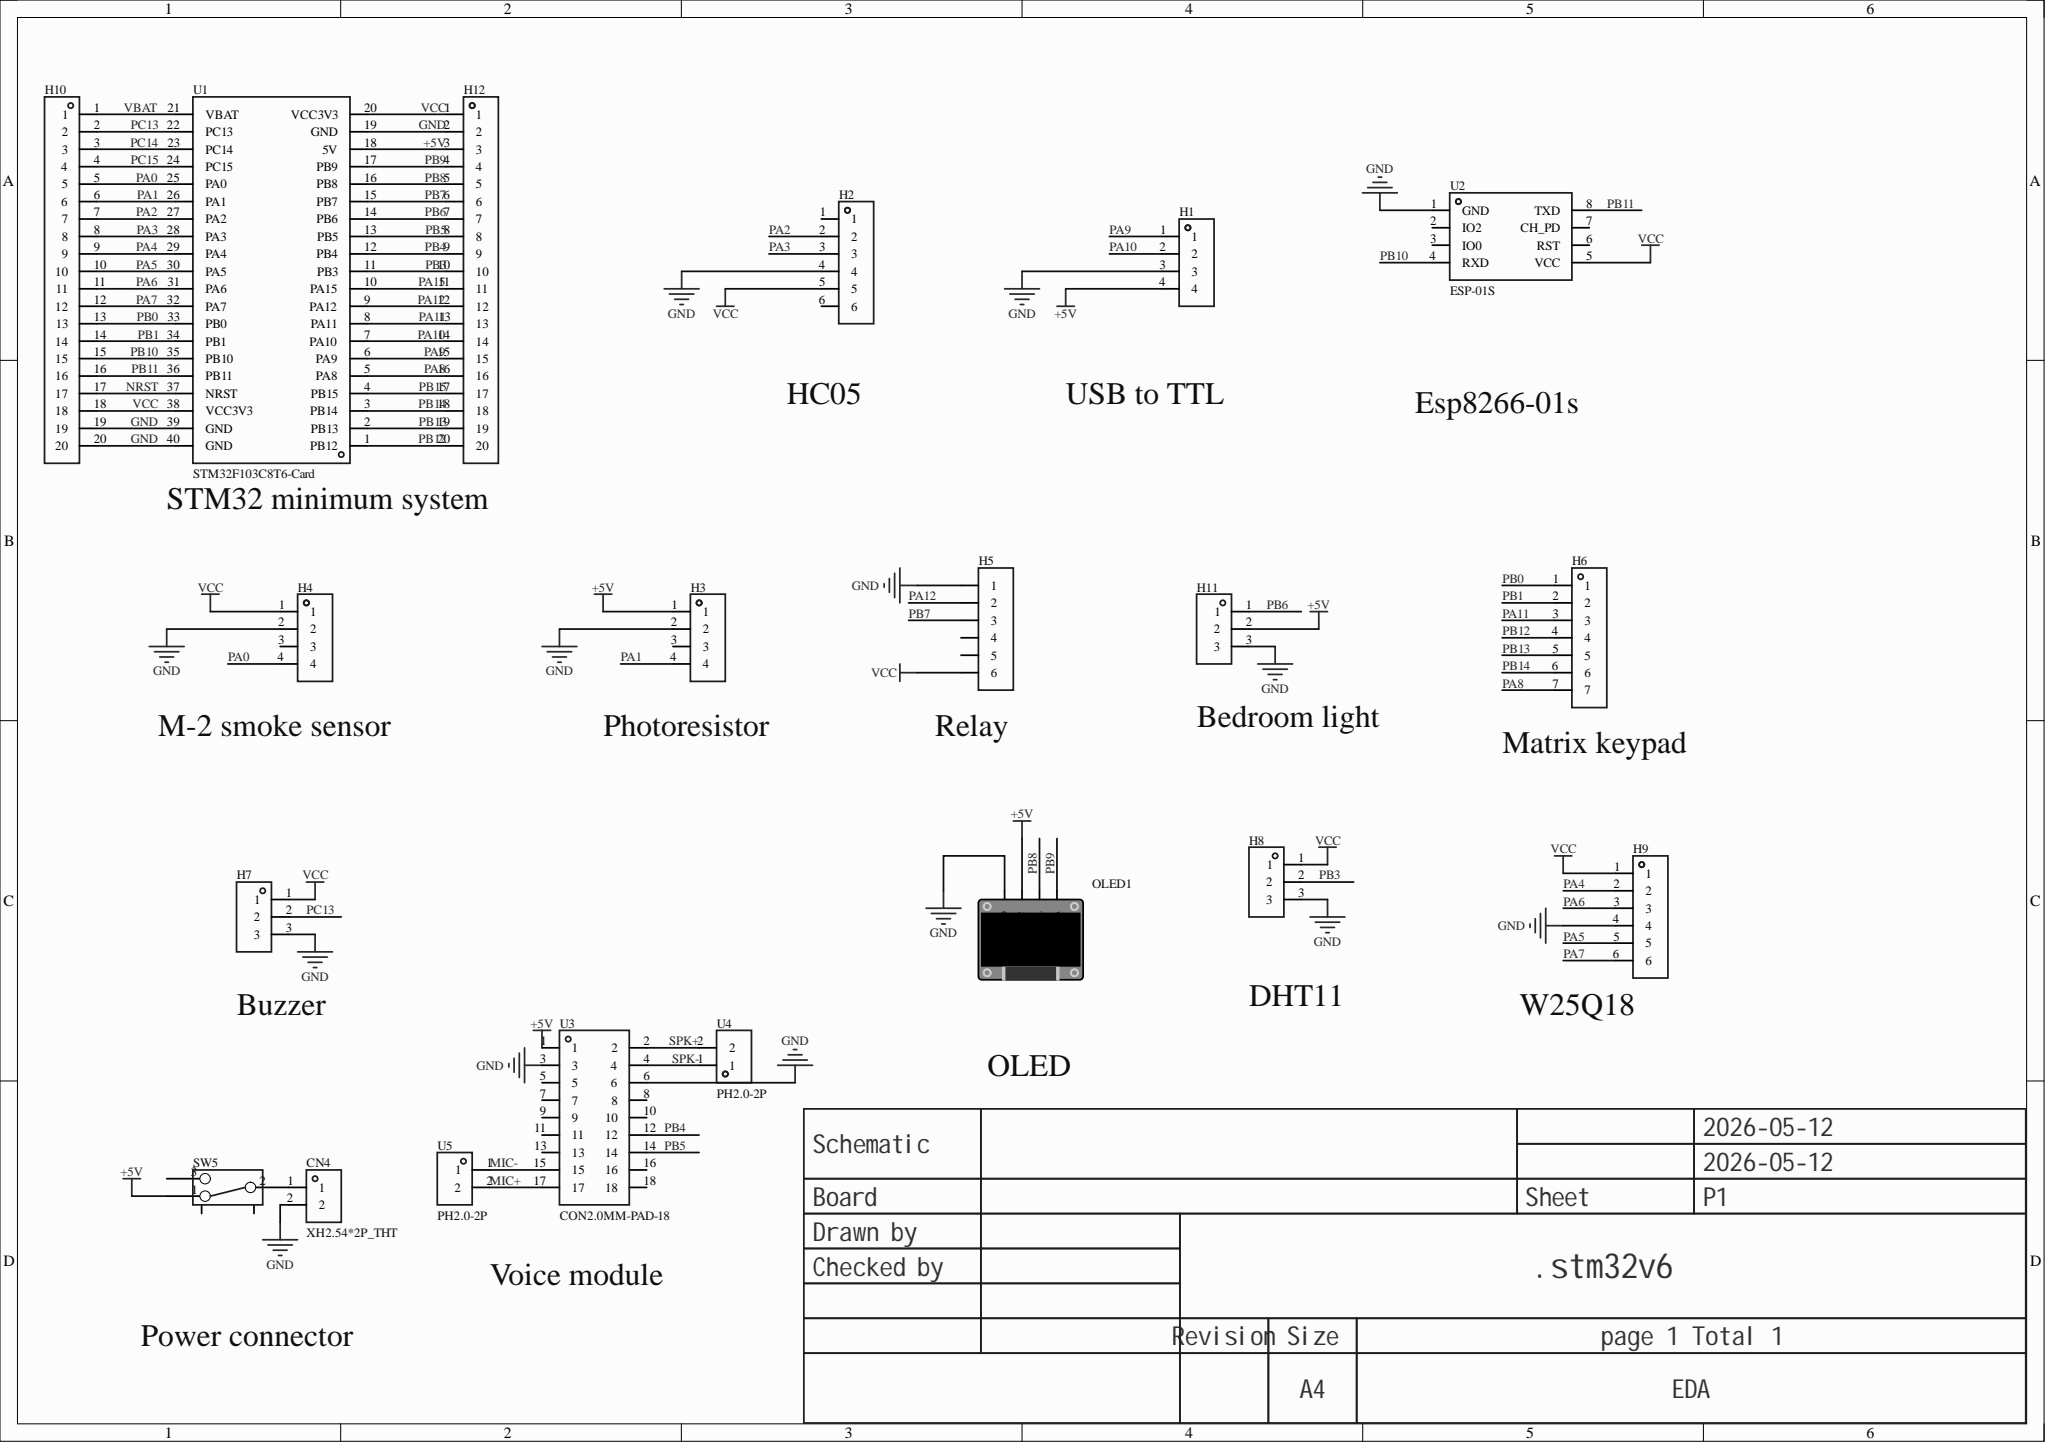Circuit board | Altium Designer | 20 parts | 42 nets
Bill of materials:
Comment,Description,Designator,Footprint,LibRef,Quantity
"XH2.54*2P_THT","","CN4","CONN-TH_2P-P2.50-XH2.54-2P","XH2.54*2P_直插","1"
"","","H1, H3, H4","HDR-TH_4P-P2.54-V-F","HDR-F_2.54_1x4P","3"
"","","H2, H9","HDR-TH_6P-P2.54-V-F","HDR-F_2.54_1x6P","2"
"","","H5","HDR-TH_6P-P2.54-V-M-1","HDR-M_2.54_1x6P","1"
"","","H6","HDR-TH_7P-P2.54-V-M","HDR-M_2.54_1x7P","1"
"","","H7, H8, H11","HDR-TH_3P-P2.54-V-F","HDR-F_2.54_1x3P","3"
"","间距:2.54mm;总PIN位数:20;排数:1;插针结构:-;行距:-;安装类型:直插;圆针/方针:-;额定电流:-;额定电压:-;配合针长度:-;塑高:-;触头材质:黄铜;触头镀层:-;颜色:黑色;","H10, H12","HDR-TH_20P-P2.54-V-M-1","HDR-M_2.54_1x20P","2"
"","","OLED1","0.96OLED_4P","0.96OLED模块_4P","1"
"","","SW5","拨动开关","拨动开关_正","1"
"STM32F103C8T6-Card","","U1","CONN-TH_L53.3-W22.9_STM32F103C8T6-CARD","STM32F103C8T6-Card","1"
"ESP-01S","","U2","WIFIM-TH_ESP-01S","ESP-01S_C111009","1"
"CON2.0MM-PAD-18","","U3","CONN-TH_18P-P2.00_C9900078766","CON2.0MM-PAD-18","1"
"PH2.0-2P","","U4, U5","CONN-TH_2P-P2.00_BOSSIE_BX-PH2.0-2PZZ","PH2.0-2P","2"
Netlist (Protel format):
[
CN4
CONN-TH_2P-P2.50-XH2.54-2P
XH2.54*2P_THT



]
[
H1
HDR-TH_4P-P2.54-V-F




]
[
H2
HDR-TH_6P-P2.54-V-F




]
[
H3
HDR-TH_4P-P2.54-V-F




]
[
H4
HDR-TH_4P-P2.54-V-F




]
[
H5
HDR-TH_6P-P2.54-V-M-1




]
[
H6
HDR-TH_7P-P2.54-V-M




]
[
H7
HDR-TH_3P-P2.54-V-F




]
[
H8
HDR-TH_3P-P2.54-V-F




]
[
H9
HDR-TH_6P-P2.54-V-F




]
[
H10
HDR-TH_20P-P2.54-V-M-1




]
[
H11
HDR-TH_3P-P2.54-V-F




]
[
H12
HDR-TH_20P-P2.54-V-M-1




]
[
OLED1
0.96OLED_4P




]
[
SW5
拨动开关




]
[
U1
CONN-TH_L53.3-W22.9_STM32F103C8T6-CARD
STM32F103C8T6-Card



]
[
U2
WIFIM-TH_ESP-01S
ESP-01S



]
[
U3
CONN-TH_18P-P2.00_C9900078766
CON2.0MM-PAD-18



]
[
U4
CONN-TH_2P-P2.00_BOSSIE_BX-PH2.0-2PZZ
PH2.0-2P



]
[
U5
CONN-TH_2P-P2.00_BOSSIE_BX-PH2.0-2PZZ
PH2.0-2P



]
(
VCC
H2-5
H4-1
H5-6
H7-1
H8-1
H9-1
H10-18
H12-1
U1-20
U1-38
U2-5
)
(
VBAT
H10-1
U1-21
)
(
SPK-
U3-4
U4-1
)
(
SPK+
U3-2
U4-2
)
(
PC15
H10-4
U1-24
)
(
PC14
H10-3
U1-23
)
(
PC13
H7-2
H10-2
U1-22
)
(
PB15
H12-17
U1-4
)
(
PB14
H6-6
H12-18
U1-3
)
(
PB13
H6-5
H12-19
U1-2
)
(
PB12
H6-4
H12-20
U1-1
)
(
PB11
H10-16
U1-36
U2-8
)
(
PB10
H10-15
U1-35
U2-4
)
(
PB9
H12-4
OLED1-4
U1-17
)
(
PB8
H12-5
OLED1-3
U1-16
)
(
PB7
H5-3
H12-6
U1-15
)
(
PB6
H11-1
H12-7
U1-14
)
(
PB5
H12-8
U1-13
U3-14
)
(
PB4
H12-9
U1-12
U3-12
)
(
PB3
H8-2
H12-10
U1-11
)
(
PB1
H6-2
H10-14
U1-34
)
(
PB0
H6-1
H10-13
U1-33
)
(
PA15
H12-11
U1-10
)
(
PA12
H5-2
H12-12
U1-9
)
(
PA11
H6-3
H12-13
U1-8
)
(
PA10
H1-2
H12-14
U1-7
)
(
PA9
H1-1
H12-15
U1-6
)
(
PA8
H6-7
H12-16
U1-5
)
(
PA7
H9-6
H10-12
U1-32
)
(
PA6
H9-3
H10-11
U1-31
)
(
PA5
H9-5
H10-10
U1-30
)
(
PA4
H9-2
H10-9
U1-29
)
(
PA3
H2-3
H10-8
U1-28
)
(
PA2
H2-2
H10-7
U1-27
)
(
PA1
H3-4
H10-6
U1-26
)
(
PA0
H4-4
H10-5
U1-25
)
(
NRST
H10-17
U1-37
)
(
NetCN4_1
CN4-1
SW5-2
)
(
MIC-
U3-15
U5-1
)
(
MIC+
U3-17
U5-2
)
(
GND
CN4-2
H1-3
H2-4
H3-2
H4-2
H5-1
H7-3
H8-3
H9-4
H10-19
H10-20
H11-3
H12-2
OLED1-1
U1-19
U1-39
U1-40
U2-1
U3-3
U3-6
)
(
+5V
H1-4
H3-1
H11-2
H12-3
OLED1-2
SW5-1
U1-18
U3-1
)